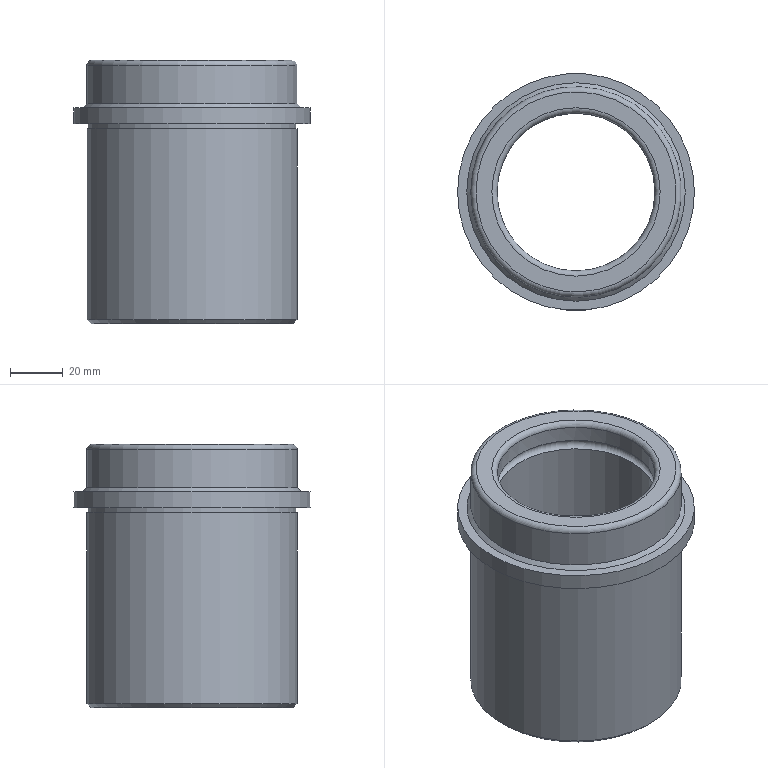Part | NX | features solid 2 | 1 solid | 21 faces | box 90 x 90 x 100 mm | volume 223284 mm3 | cylinder 8 | plane 5 | torus 4 | cone 4 | commonest cylinder face diameters 60 x3 80 x2 61 x1 79 x1 90 x1
STEP:
#1=CARTESIAN_POINT('',(380.,350.,152.5));
#2=VERTEX_POINT('',#1);
#3=CARTESIAN_POINT('',(340.,350.,152.5));
#4=DIRECTION('',(0.,0.,1.));
#5=DIRECTION('',(1.,0.,0.));
#6=AXIS2_PLACEMENT_3D('',#3,#4,#5);
#7=CIRCLE('',#6,40.);
#8=EDGE_CURVE('',#2,#2,#7,.F.);
#9=ORIENTED_EDGE('',*,*,#8,.F.);
#10=EDGE_LOOP('',(#9));
#11=FACE_BOUND('',#10,.T.);
#12=CARTESIAN_POINT('',(380.,350.,225.));
#13=VERTEX_POINT('',#12);
#14=CARTESIAN_POINT('',(340.,350.,225.));
#15=DIRECTION('',(0.,0.,1.));
#16=DIRECTION('',(1.,0.,0.));
#17=AXIS2_PLACEMENT_3D('',#14,#15,#16);
#18=CIRCLE('',#17,40.);
#19=EDGE_CURVE('',#13,#13,#18,.T.);
#20=ORIENTED_EDGE('',*,*,#19,.F.);
#21=EDGE_LOOP('',(#20));
#22=FACE_BOUND('',#21,.T.);
#23=CARTESIAN_POINT('',(340.,350.,169.813));
#24=DIRECTION('',(0.,0.,-1.));
#25=DIRECTION('',(1.,0.,0.));
#26=AXIS2_PLACEMENT_3D('',#23,#24,#25);
#27=CYLINDRICAL_SURFACE('',#26,40.);
#28=ADVANCED_FACE('',(#11,#22),#27,.T.);
#29=CARTESIAN_POINT('',(379.5,350.,225.));
#30=VERTEX_POINT('',#29);
#31=CARTESIAN_POINT('',(340.,350.,225.));
#32=DIRECTION('',(0.,0.,1.));
#33=DIRECTION('',(1.,0.,0.));
#34=AXIS2_PLACEMENT_3D('',#31,#32,#33);
#35=CIRCLE('',#34,39.5);
#36=EDGE_CURVE('',#30,#30,#35,.T.);
#37=ORIENTED_EDGE('',*,*,#36,.F.);
#38=EDGE_LOOP('',(#37));
#39=FACE_BOUND('',#38,.T.);
#40=ORIENTED_EDGE('',*,*,#19,.T.);
#41=EDGE_LOOP('',(#40));
#42=FACE_BOUND('',#41,.T.);
#43=CARTESIAN_POINT('',(340.,310.,225.));
#44=DIRECTION('',(0.,0.,1.));
#45=DIRECTION('',(-1.,0.,0.));
#46=AXIS2_PLACEMENT_3D('',#43,#44,#45);
#47=PLANE('',#46);
#48=ADVANCED_FACE('',(#39,#42),#47,.T.);
#49=CARTESIAN_POINT('',(379.5,350.,227.));
#50=VERTEX_POINT('',#49);
#51=CARTESIAN_POINT('',(340.,350.,227.));
#52=DIRECTION('',(0.,0.,1.));
#53=DIRECTION('',(1.,0.,0.));
#54=AXIS2_PLACEMENT_3D('',#51,#52,#53);
#55=CIRCLE('',#54,39.5);
#56=EDGE_CURVE('',#50,#50,#55,.T.);
#57=ORIENTED_EDGE('',*,*,#56,.F.);
#58=EDGE_LOOP('',(#57));
#59=FACE_BOUND('',#58,.T.);
#60=ORIENTED_EDGE('',*,*,#36,.T.);
#61=EDGE_LOOP('',(#60));
#62=FACE_BOUND('',#61,.T.);
#63=CARTESIAN_POINT('',(340.,350.,169.813));
#64=DIRECTION('',(0.,0.,-1.));
#65=DIRECTION('',(1.,0.,0.));
#66=AXIS2_PLACEMENT_3D('',#63,#64,#65);
#67=CYLINDRICAL_SURFACE('',#66,39.5);
#68=ADVANCED_FACE('',(#59,#62),#67,.T.);
#69=CARTESIAN_POINT('',(385.,350.,227.));
#70=VERTEX_POINT('',#69);
#71=CARTESIAN_POINT('',(340.,350.,227.));
#72=DIRECTION('',(0.,0.,1.));
#73=DIRECTION('',(1.,0.,0.));
#74=AXIS2_PLACEMENT_3D('',#71,#72,#73);
#75=CIRCLE('',#74,45.);
#76=EDGE_CURVE('',#70,#70,#75,.T.);
#77=ORIENTED_EDGE('',*,*,#76,.F.);
#78=EDGE_LOOP('',(#77));
#79=FACE_BOUND('',#78,.T.);
#80=ORIENTED_EDGE('',*,*,#56,.T.);
#81=EDGE_LOOP('',(#80));
#82=FACE_BOUND('',#81,.T.);
#83=CARTESIAN_POINT('',(340.,310.5,227.));
#84=DIRECTION('',(0.,0.,-1.));
#85=DIRECTION('',(1.,0.,0.));
#86=AXIS2_PLACEMENT_3D('',#83,#84,#85);
#87=PLANE('',#86);
#88=ADVANCED_FACE('',(#79,#82),#87,.T.);
#89=CARTESIAN_POINT('',(385.,350.,233.));
#90=VERTEX_POINT('',#89);
#91=CARTESIAN_POINT('',(340.,350.,233.));
#92=DIRECTION('',(0.,0.,1.));
#93=DIRECTION('',(1.,0.,0.));
#94=AXIS2_PLACEMENT_3D('',#91,#92,#93);
#95=CIRCLE('',#94,45.);
#96=EDGE_CURVE('',#90,#90,#95,.T.);
#97=ORIENTED_EDGE('',*,*,#96,.F.);
#98=EDGE_LOOP('',(#97));
#99=FACE_BOUND('',#98,.T.);
#100=ORIENTED_EDGE('',*,*,#76,.T.);
#101=EDGE_LOOP('',(#100));
#102=FACE_BOUND('',#101,.T.);
#103=CARTESIAN_POINT('',(340.,350.,169.813));
#104=DIRECTION('',(0.,0.,-1.));
#105=DIRECTION('',(1.,0.,0.));
#106=AXIS2_PLACEMENT_3D('',#103,#104,#105);
#107=CYLINDRICAL_SURFACE('',#106,45.);
#108=ADVANCED_FACE('',(#99,#102),#107,.T.);
#109=CARTESIAN_POINT('',(298.5,350.,233.));
#110=VERTEX_POINT('',#109);
#111=CARTESIAN_POINT('',(340.,350.,233.));
#112=DIRECTION('',(0.,0.,-1.));
#113=DIRECTION('',(-1.,0.,0.));
#114=AXIS2_PLACEMENT_3D('',#111,#112,#113);
#115=CIRCLE('',#114,41.5);
#116=EDGE_CURVE('',#110,#110,#115,.F.);
#117=ORIENTED_EDGE('',*,*,#116,.F.);
#118=EDGE_LOOP('',(#117));
#119=FACE_BOUND('',#118,.T.);
#120=ORIENTED_EDGE('',*,*,#96,.T.);
#121=EDGE_LOOP('',(#120));
#122=FACE_BOUND('',#121,.T.);
#123=CARTESIAN_POINT('',(340.,305.,233.));
#124=DIRECTION('',(0.,0.,1.));
#125=DIRECTION('',(-1.,0.,0.));
#126=AXIS2_PLACEMENT_3D('',#123,#124,#125);
#127=PLANE('',#126);
#128=ADVANCED_FACE('',(#119,#122),#127,.T.);
#129=CARTESIAN_POINT('',(300.,350.,249.));
#130=VERTEX_POINT('',#129);
#131=CARTESIAN_POINT('',(340.,350.,249.));
#132=DIRECTION('',(0.,0.,-1.));
#133=DIRECTION('',(-1.,0.,0.));
#134=AXIS2_PLACEMENT_3D('',#131,#132,#133);
#135=CIRCLE('',#134,40.);
#136=EDGE_CURVE('',#130,#130,#135,.F.);
#137=ORIENTED_EDGE('',*,*,#136,.F.);
#138=EDGE_LOOP('',(#137));
#139=FACE_BOUND('',#138,.T.);
#140=CARTESIAN_POINT('',(300.,350.,234.5));
#141=VERTEX_POINT('',#140);
#142=CARTESIAN_POINT('',(340.,350.,234.5));
#143=DIRECTION('',(0.,0.,-1.));
#144=DIRECTION('',(-1.,0.,0.));
#145=AXIS2_PLACEMENT_3D('',#142,#143,#144);
#146=CIRCLE('',#145,40.);
#147=EDGE_CURVE('',#141,#141,#146,.T.);
#148=ORIENTED_EDGE('',*,*,#147,.F.);
#149=EDGE_LOOP('',(#148));
#150=FACE_BOUND('',#149,.T.);
#151=CARTESIAN_POINT('',(340.,350.,169.813));
#152=DIRECTION('',(0.,0.,-1.));
#153=DIRECTION('',(1.,0.,0.));
#154=AXIS2_PLACEMENT_3D('',#151,#152,#153);
#155=CYLINDRICAL_SURFACE('',#154,40.);
#156=ADVANCED_FACE('',(#139,#150),#155,.T.);
#157=CARTESIAN_POINT('',(302.,350.,251.));
#158=VERTEX_POINT('',#157);
#159=CARTESIAN_POINT('',(340.,350.,251.));
#160=DIRECTION('',(0.,0.,-1.));
#161=DIRECTION('',(-1.,0.,0.));
#162=AXIS2_PLACEMENT_3D('',#159,#160,#161);
#163=CIRCLE('',#162,38.);
#164=EDGE_CURVE('',#158,#158,#163,.T.);
#165=ORIENTED_EDGE('',*,*,#164,.F.);
#166=EDGE_LOOP('',(#165));
#167=FACE_BOUND('',#166,.T.);
#168=CARTESIAN_POINT('',(308.,350.,251.));
#169=VERTEX_POINT('',#168);
#170=CARTESIAN_POINT('',(340.,350.,251.));
#171=DIRECTION('',(0.,0.,-1.));
#172=DIRECTION('',(-1.,0.,0.));
#173=AXIS2_PLACEMENT_3D('',#170,#171,#172);
#174=CIRCLE('',#173,32.);
#175=EDGE_CURVE('',#169,#169,#174,.F.);
#176=ORIENTED_EDGE('',*,*,#175,.F.);
#177=EDGE_LOOP('',(#176));
#178=FACE_BOUND('',#177,.T.);
#179=CARTESIAN_POINT('',(340.,310.,251.));
#180=DIRECTION('',(0.,0.,1.));
#181=DIRECTION('',(-1.,0.,0.));
#182=AXIS2_PLACEMENT_3D('',#179,#180,#181);
#183=PLANE('',#182);
#184=ADVANCED_FACE('',(#167,#178),#183,.T.);
#185=CARTESIAN_POINT('',(310.,350.,249.));
#186=VERTEX_POINT('',#185);
#187=CARTESIAN_POINT('',(340.,350.,249.));
#188=DIRECTION('',(0.,0.,-1.));
#189=DIRECTION('',(-1.,0.,0.));
#190=AXIS2_PLACEMENT_3D('',#187,#188,#189);
#191=CIRCLE('',#190,30.);
#192=EDGE_CURVE('',#186,#186,#191,.T.);
#193=ORIENTED_EDGE('',*,*,#192,.F.);
#194=EDGE_LOOP('',(#193));
#195=FACE_BOUND('',#194,.T.);
#196=CARTESIAN_POINT('',(370.,350.,242.973));
#197=VERTEX_POINT('',#196);
#198=CARTESIAN_POINT('',(340.,350.,242.973));
#199=DIRECTION('',(0.,0.,1.));
#200=DIRECTION('',(1.,0.,0.));
#201=AXIS2_PLACEMENT_3D('',#198,#199,#200);
#202=CIRCLE('',#201,30.);
#203=EDGE_CURVE('',#197,#197,#202,.T.);
#204=ORIENTED_EDGE('',*,*,#203,.F.);
#205=EDGE_LOOP('',(#204));
#206=FACE_BOUND('',#205,.T.);
#207=CARTESIAN_POINT('',(340.,350.,169.813));
#208=DIRECTION('',(0.,0.,-1.));
#209=DIRECTION('',(1.,0.,0.));
#210=AXIS2_PLACEMENT_3D('',#207,#208,#209);
#211=CYLINDRICAL_SURFACE('',#210,30.);
#212=ADVANCED_FACE('',(#195,#206),#211,.F.);
#213=ORIENTED_EDGE('',*,*,#203,.T.);
#214=EDGE_LOOP('',(#213));
#215=FACE_BOUND('',#214,.T.);
#216=CARTESIAN_POINT('',(370.,350.,239.027));
#217=VERTEX_POINT('',#216);
#218=CARTESIAN_POINT('',(340.,350.,239.027));
#219=DIRECTION('',(0.,0.,1.));
#220=DIRECTION('',(1.,0.,0.));
#221=AXIS2_PLACEMENT_3D('',#218,#219,#220);
#222=CIRCLE('',#221,30.);
#223=EDGE_CURVE('',#217,#217,#222,.T.);
#224=ORIENTED_EDGE('',*,*,#223,.F.);
#225=EDGE_LOOP('',(#224));
#226=FACE_BOUND('',#225,.T.);
#227=CARTESIAN_POINT('',(340.,350.,241.));
#228=DIRECTION('',(0.,0.,-1.));
#229=DIRECTION('',(1.,0.,0.));
#230=AXIS2_PLACEMENT_3D('',#227,#228,#229);
#231=TOROIDAL_SURFACE('',#230,29.674,2.);
#232=ADVANCED_FACE('',(#215,#226),#231,.F.);
#233=CARTESIAN_POINT('',(370.,350.,207.973));
#234=VERTEX_POINT('',#233);
#235=CARTESIAN_POINT('',(340.,350.,207.973));
#236=DIRECTION('',(0.,0.,1.));
#237=DIRECTION('',(1.,0.,0.));
#238=AXIS2_PLACEMENT_3D('',#235,#236,#237);
#239=CIRCLE('',#238,30.);
#240=EDGE_CURVE('',#234,#234,#239,.T.);
#241=ORIENTED_EDGE('',*,*,#240,.F.);
#242=EDGE_LOOP('',(#241));
#243=FACE_BOUND('',#242,.T.);
#244=ORIENTED_EDGE('',*,*,#223,.T.);
#245=EDGE_LOOP('',(#244));
#246=FACE_BOUND('',#245,.T.);
#247=CARTESIAN_POINT('',(340.,350.,169.813));
#248=DIRECTION('',(0.,0.,-1.));
#249=DIRECTION('',(1.,0.,0.));
#250=AXIS2_PLACEMENT_3D('',#247,#248,#249);
#251=CYLINDRICAL_SURFACE('',#250,30.);
#252=ADVANCED_FACE('',(#243,#246),#251,.F.);
#253=ORIENTED_EDGE('',*,*,#240,.T.);
#254=EDGE_LOOP('',(#253));
#255=FACE_BOUND('',#254,.T.);
#256=CARTESIAN_POINT('',(370.,350.,204.027));
#257=VERTEX_POINT('',#256);
#258=CARTESIAN_POINT('',(340.,350.,204.027));
#259=DIRECTION('',(0.,0.,1.));
#260=DIRECTION('',(1.,0.,0.));
#261=AXIS2_PLACEMENT_3D('',#258,#259,#260);
#262=CIRCLE('',#261,30.);
#263=EDGE_CURVE('',#257,#257,#262,.T.);
#264=ORIENTED_EDGE('',*,*,#263,.F.);
#265=EDGE_LOOP('',(#264));
#266=FACE_BOUND('',#265,.T.);
#267=CARTESIAN_POINT('',(340.,350.,206.));
#268=DIRECTION('',(0.,0.,-1.));
#269=DIRECTION('',(1.,0.,0.));
#270=AXIS2_PLACEMENT_3D('',#267,#268,#269);
#271=TOROIDAL_SURFACE('',#270,29.674,2.);
#272=ADVANCED_FACE('',(#255,#266),#271,.F.);
#273=CARTESIAN_POINT('',(370.,350.,171.));
#274=VERTEX_POINT('',#273);
#275=CARTESIAN_POINT('',(340.,350.,171.));
#276=DIRECTION('',(0.,0.,1.));
#277=DIRECTION('',(1.,0.,0.));
#278=AXIS2_PLACEMENT_3D('',#275,#276,#277);
#279=CIRCLE('',#278,30.);
#280=EDGE_CURVE('',#274,#274,#279,.T.);
#281=ORIENTED_EDGE('',*,*,#280,.F.);
#282=EDGE_LOOP('',(#281));
#283=FACE_BOUND('',#282,.T.);
#284=ORIENTED_EDGE('',*,*,#263,.T.);
#285=EDGE_LOOP('',(#284));
#286=FACE_BOUND('',#285,.T.);
#287=CARTESIAN_POINT('',(340.,350.,169.813));
#288=DIRECTION('',(0.,0.,-1.));
#289=DIRECTION('',(1.,0.,0.));
#290=AXIS2_PLACEMENT_3D('',#287,#288,#289);
#291=CYLINDRICAL_SURFACE('',#290,30.);
#292=ADVANCED_FACE('',(#283,#286),#291,.F.);
#293=CARTESIAN_POINT('',(370.5,350.,170.5));
#294=VERTEX_POINT('',#293);
#295=CARTESIAN_POINT('',(340.,350.,170.5));
#296=DIRECTION('',(0.,0.,1.));
#297=DIRECTION('',(1.,0.,0.));
#298=AXIS2_PLACEMENT_3D('',#295,#296,#297);
#299=CIRCLE('',#298,30.5);
#300=EDGE_CURVE('',#294,#294,#299,.T.);
#301=ORIENTED_EDGE('',*,*,#300,.F.);
#302=EDGE_LOOP('',(#301));
#303=FACE_BOUND('',#302,.T.);
#304=ORIENTED_EDGE('',*,*,#280,.T.);
#305=EDGE_LOOP('',(#304));
#306=FACE_BOUND('',#305,.T.);
#307=CARTESIAN_POINT('',(340.,350.,171.));
#308=DIRECTION('',(0.,0.,-1.));
#309=DIRECTION('',(1.,0.,0.));
#310=AXIS2_PLACEMENT_3D('',#307,#308,#309);
#311=CONICAL_SURFACE('',#310,30.,0.7854);
#312=ADVANCED_FACE('',(#303,#306),#311,.F.);
#313=CARTESIAN_POINT('',(370.5,350.,152.5));
#314=VERTEX_POINT('',#313);
#315=CARTESIAN_POINT('',(340.,350.,152.5));
#316=DIRECTION('',(0.,0.,1.));
#317=DIRECTION('',(1.,0.,0.));
#318=AXIS2_PLACEMENT_3D('',#315,#316,#317);
#319=CIRCLE('',#318,30.5);
#320=EDGE_CURVE('',#314,#314,#319,.T.);
#321=ORIENTED_EDGE('',*,*,#320,.F.);
#322=EDGE_LOOP('',(#321));
#323=FACE_BOUND('',#322,.T.);
#324=ORIENTED_EDGE('',*,*,#300,.T.);
#325=EDGE_LOOP('',(#324));
#326=FACE_BOUND('',#325,.T.);
#327=CARTESIAN_POINT('',(340.,350.,169.813));
#328=DIRECTION('',(0.,0.,-1.));
#329=DIRECTION('',(1.,0.,0.));
#330=AXIS2_PLACEMENT_3D('',#327,#328,#329);
#331=CYLINDRICAL_SURFACE('',#330,30.5);
#332=ADVANCED_FACE('',(#323,#326),#331,.F.);
#333=CARTESIAN_POINT('',(372.,350.,151.));
#334=VERTEX_POINT('',#333);
#335=CARTESIAN_POINT('',(340.,350.,151.));
#336=DIRECTION('',(0.,0.,1.));
#337=DIRECTION('',(1.,0.,0.));
#338=AXIS2_PLACEMENT_3D('',#335,#336,#337);
#339=CIRCLE('',#338,32.);
#340=EDGE_CURVE('',#334,#334,#339,.F.);
#341=ORIENTED_EDGE('',*,*,#340,.F.);
#342=EDGE_LOOP('',(#341));
#343=FACE_BOUND('',#342,.T.);
#344=CARTESIAN_POINT('',(378.5,350.,151.));
#345=VERTEX_POINT('',#344);
#346=CARTESIAN_POINT('',(340.,350.,151.));
#347=DIRECTION('',(0.,0.,1.));
#348=DIRECTION('',(1.,0.,0.));
#349=AXIS2_PLACEMENT_3D('',#346,#347,#348);
#350=CIRCLE('',#349,38.5);
#351=EDGE_CURVE('',#345,#345,#350,.T.);
#352=ORIENTED_EDGE('',*,*,#351,.F.);
#353=EDGE_LOOP('',(#352));
#354=FACE_BOUND('',#353,.T.);
#355=CARTESIAN_POINT('',(340.,319.5,151.));
#356=DIRECTION('',(0.,0.,-1.));
#357=DIRECTION('',(1.,0.,0.));
#358=AXIS2_PLACEMENT_3D('',#355,#356,#357);
#359=PLANE('',#358);
#360=ADVANCED_FACE('',(#343,#354),#359,.T.);
#361=ORIENTED_EDGE('',*,*,#340,.T.);
#362=EDGE_LOOP('',(#361));
#363=FACE_BOUND('',#362,.T.);
#364=ORIENTED_EDGE('',*,*,#320,.T.);
#365=EDGE_LOOP('',(#364));
#366=FACE_BOUND('',#365,.T.);
#367=CARTESIAN_POINT('',(340.,350.,152.5));
#368=DIRECTION('',(0.,0.,-1.));
#369=DIRECTION('',(1.,0.,0.));
#370=AXIS2_PLACEMENT_3D('',#367,#368,#369);
#371=CONICAL_SURFACE('',#370,30.5,0.7854);
#372=ADVANCED_FACE('',(#363,#366),#371,.F.);
#373=ORIENTED_EDGE('',*,*,#8,.T.);
#374=EDGE_LOOP('',(#373));
#375=FACE_BOUND('',#374,.T.);
#376=ORIENTED_EDGE('',*,*,#351,.T.);
#377=EDGE_LOOP('',(#376));
#378=FACE_BOUND('',#377,.T.);
#379=CARTESIAN_POINT('',(340.,350.,151.));
#380=DIRECTION('',(0.,0.,1.));
#381=DIRECTION('',(-1.,0.,0.));
#382=AXIS2_PLACEMENT_3D('',#379,#380,#381);
#383=CONICAL_SURFACE('',#382,38.5,0.7854);
#384=ADVANCED_FACE('',(#375,#378),#383,.T.);
#385=ORIENTED_EDGE('',*,*,#147,.T.);
#386=EDGE_LOOP('',(#385));
#387=FACE_BOUND('',#386,.T.);
#388=ORIENTED_EDGE('',*,*,#116,.T.);
#389=EDGE_LOOP('',(#388));
#390=FACE_BOUND('',#389,.T.);
#391=CARTESIAN_POINT('',(340.,350.,233.));
#392=DIRECTION('',(0.,0.,-1.));
#393=DIRECTION('',(1.,0.,0.));
#394=AXIS2_PLACEMENT_3D('',#391,#392,#393);
#395=CONICAL_SURFACE('',#394,41.5,0.7854);
#396=ADVANCED_FACE('',(#387,#390),#395,.T.);
#397=ORIENTED_EDGE('',*,*,#164,.T.);
#398=EDGE_LOOP('',(#397));
#399=FACE_BOUND('',#398,.T.);
#400=ORIENTED_EDGE('',*,*,#136,.T.);
#401=EDGE_LOOP('',(#400));
#402=FACE_BOUND('',#401,.T.);
#403=CARTESIAN_POINT('',(340.,350.,249.));
#404=DIRECTION('',(0.,0.,1.));
#405=DIRECTION('',(-1.,0.,0.));
#406=AXIS2_PLACEMENT_3D('',#403,#404,#405);
#407=TOROIDAL_SURFACE('',#406,38.,2.);
#408=ADVANCED_FACE('',(#399,#402),#407,.T.);
#409=ORIENTED_EDGE('',*,*,#192,.T.);
#410=EDGE_LOOP('',(#409));
#411=FACE_BOUND('',#410,.T.);
#412=ORIENTED_EDGE('',*,*,#175,.T.);
#413=EDGE_LOOP('',(#412));
#414=FACE_BOUND('',#413,.T.);
#415=CARTESIAN_POINT('',(340.,350.,249.));
#416=DIRECTION('',(0.,0.,1.));
#417=DIRECTION('',(-1.,0.,0.));
#418=AXIS2_PLACEMENT_3D('',#415,#416,#417);
#419=TOROIDAL_SURFACE('',#418,32.,2.);
#420=ADVANCED_FACE('',(#411,#414),#419,.T.);
#421=CLOSED_SHELL('',(#28,#48,#68,#88,#108,#128,#156,#184,#212,#232,#252,#272,#292,#312,#332,#360,#372,#384,#396,#408,#420));
#422=MANIFOLD_SOLID_BREP('',#421);
#423=(LENGTH_UNIT()NAMED_UNIT(*)SI_UNIT(.MILLI.,.METRE.));
#424=UNCERTAINTY_MEASURE_WITH_UNIT(LENGTH_MEASURE(0.00001),#423,'','');
#425=(NAMED_UNIT(*)PLANE_ANGLE_UNIT()SI_UNIT($,.RADIAN.));
#426=(NAMED_UNIT(*)SI_UNIT($,.STERADIAN.)SOLID_ANGLE_UNIT());
#427=(GEOMETRIC_REPRESENTATION_CONTEXT(3)GLOBAL_UNCERTAINTY_ASSIGNED_CONTEXT((#424))GLOBAL_UNIT_ASSIGNED_CONTEXT((#423,#425,#426))REPRESENTATION_CONTEXT('',''));
#428=ADVANCED_BREP_SHAPE_REPRESENTATION('',(#422),#427);